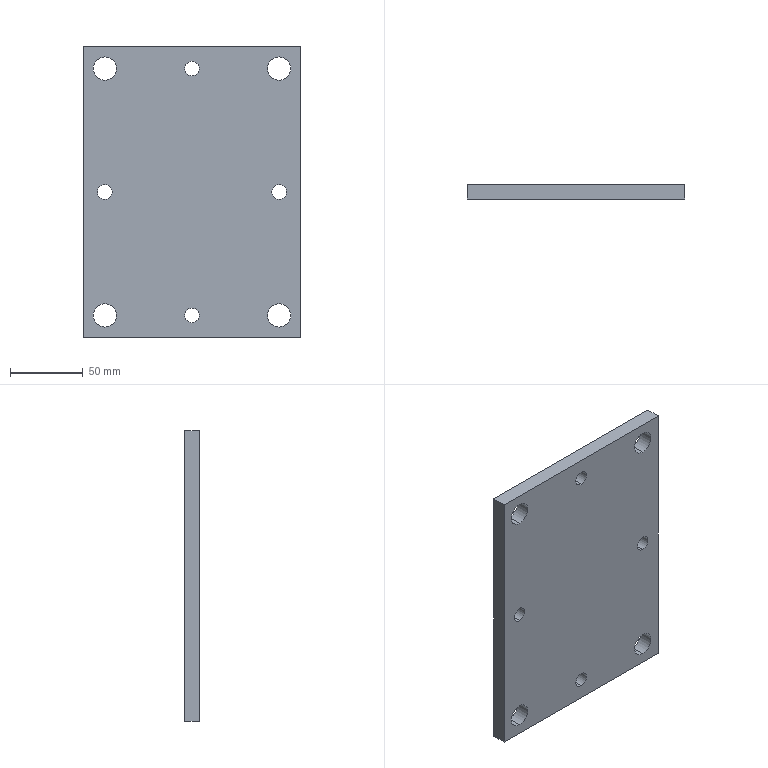Part | STEP file | E3-楼梯立柱底Plate 1 | 1 solid | 22 faces | box 150 x 10 x 200 mm | volume 288689 mm3 | cylinder 16 | plane 6 | commonest cylinder face diameters 10.2 x8 16 x8